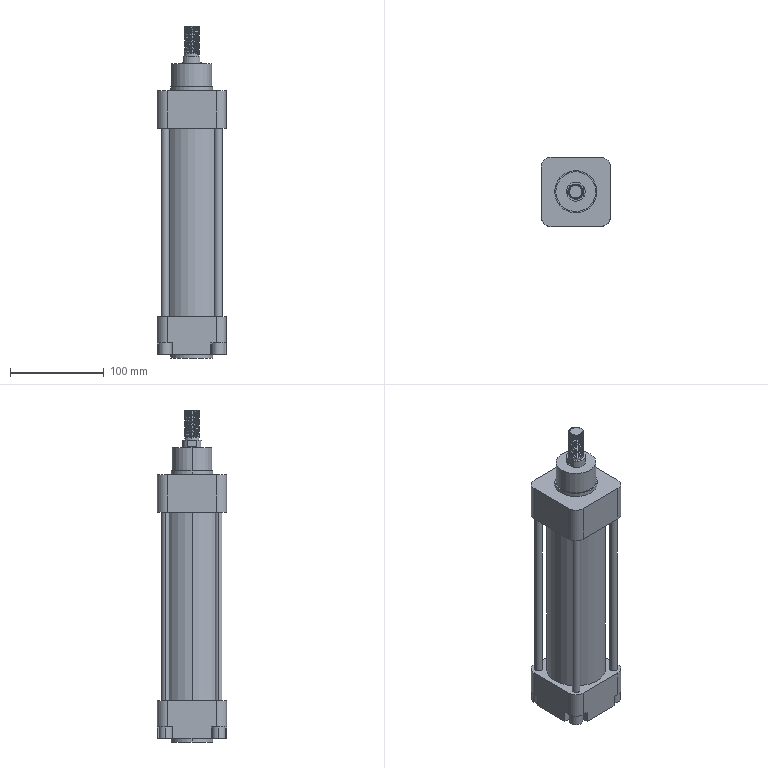Part | NX | 22 solids | 236 faces | box 74.5 x 74 x 354 mm | volume 615079 mm3 | cylinder 119 | plane 111 | cone 4 | spline 2 | commonest cylinder face diameters 16 x41 10 x12 8 x8 14 x8 21.378 x8 20 x6